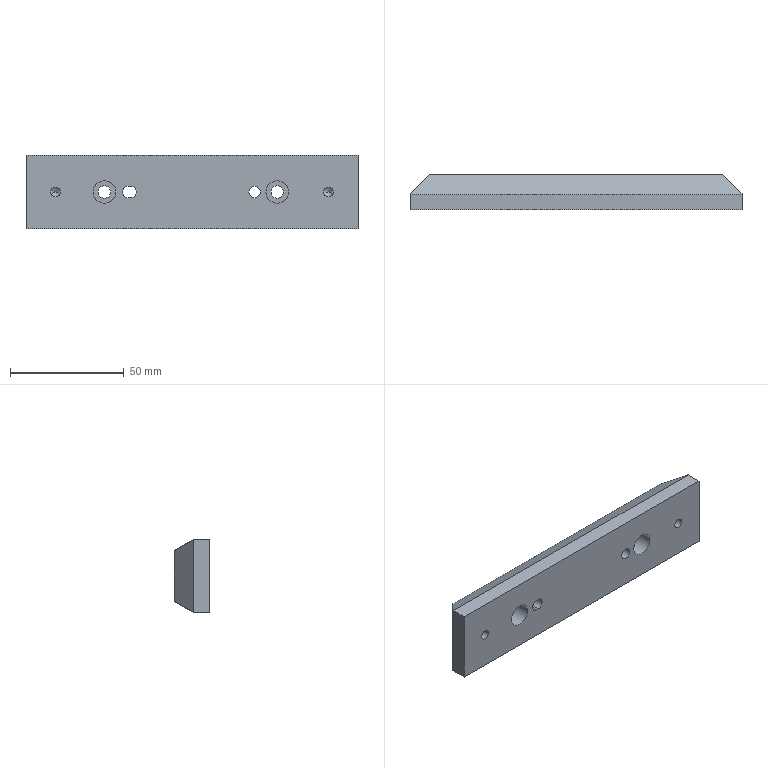Part | NX | 1 solid | 34 faces | box 146 x 15.5 x 32.5 mm | volume 62295 mm3 | cylinder 16 | plane 14 | cone 4 | commonest cylinder face diameters 4.2 x4 5 x4 5.5 x4 10 x4
STEP:
#1=CARTESIAN_POINT('',(73.,-7.75,-16.25));
#2=VERTEX_POINT('',#1);
#3=CARTESIAN_POINT('',(-73.,-7.75,-16.25));
#4=VERTEX_POINT('',#3);
#5=CARTESIAN_POINT('',(73.,-7.75,-16.25));
#6=DIRECTION('',(-1.,0.,0.));
#7=VECTOR('',#6,1000.);
#8=LINE('',#5,#7);
#9=EDGE_CURVE('',#2,#4,#8,.T.);
#10=ORIENTED_EDGE('',*,*,#9,.F.);
#11=CARTESIAN_POINT('',(73.,-7.75,16.25));
#12=VERTEX_POINT('',#11);
#13=CARTESIAN_POINT('',(73.,-7.75,16.25));
#14=DIRECTION('',(0.,0.,-1.));
#15=VECTOR('',#14,1000.);
#16=LINE('',#13,#15);
#17=EDGE_CURVE('',#12,#2,#16,.T.);
#18=ORIENTED_EDGE('',*,*,#17,.F.);
#19=CARTESIAN_POINT('',(-73.,-7.75,16.25));
#20=VERTEX_POINT('',#19);
#21=CARTESIAN_POINT('',(-73.,-7.75,16.25));
#22=DIRECTION('',(1.,0.,0.));
#23=VECTOR('',#22,1000.);
#24=LINE('',#21,#23);
#25=EDGE_CURVE('',#20,#12,#24,.T.);
#26=ORIENTED_EDGE('',*,*,#25,.F.);
#27=CARTESIAN_POINT('',(-73.,-7.75,-16.25));
#28=DIRECTION('',(0.,0.,1.));
#29=VECTOR('',#28,1000.);
#30=LINE('',#27,#29);
#31=EDGE_CURVE('',#4,#20,#30,.T.);
#32=ORIENTED_EDGE('',*,*,#31,.F.);
#33=EDGE_LOOP('',(#10,#18,#26,#32));
#34=FACE_BOUND('',#33,.T.);
#35=CARTESIAN_POINT('',(42.5,-7.75,0.));
#36=VERTEX_POINT('',#35);
#37=CARTESIAN_POINT('',(32.5,-7.75,0.));
#38=VERTEX_POINT('',#37);
#39=CARTESIAN_POINT('',(37.5,-7.75,0.));
#40=DIRECTION('',(0.,-1.,0.));
#41=DIRECTION('',(1.,0.,0.));
#42=AXIS2_PLACEMENT_3D('',#39,#40,#41);
#43=CIRCLE('',#42,5.);
#44=EDGE_CURVE('',#36,#38,#43,.T.);
#45=ORIENTED_EDGE('',*,*,#44,.F.);
#46=CARTESIAN_POINT('',(37.5,-7.75,0.));
#47=DIRECTION('',(0.,-1.,0.));
#48=DIRECTION('',(-1.,0.,0.));
#49=AXIS2_PLACEMENT_3D('',#46,#47,#48);
#50=CIRCLE('',#49,5.);
#51=EDGE_CURVE('',#38,#36,#50,.T.);
#52=ORIENTED_EDGE('',*,*,#51,.F.);
#53=EDGE_LOOP('',(#45,#52));
#54=FACE_BOUND('',#53,.T.);
#55=CARTESIAN_POINT('',(-33.5,-7.75,0.));
#56=VERTEX_POINT('',#55);
#57=CARTESIAN_POINT('',(-43.5,-7.75,0.));
#58=VERTEX_POINT('',#57);
#59=CARTESIAN_POINT('',(-38.5,-7.75,0.));
#60=DIRECTION('',(0.,-1.,0.));
#61=DIRECTION('',(1.,0.,0.));
#62=AXIS2_PLACEMENT_3D('',#59,#60,#61);
#63=CIRCLE('',#62,5.);
#64=EDGE_CURVE('',#56,#58,#63,.T.);
#65=ORIENTED_EDGE('',*,*,#64,.F.);
#66=CARTESIAN_POINT('',(-38.5,-7.75,0.));
#67=DIRECTION('',(0.,-1.,0.));
#68=DIRECTION('',(-1.,0.,0.));
#69=AXIS2_PLACEMENT_3D('',#66,#67,#68);
#70=CIRCLE('',#69,5.);
#71=EDGE_CURVE('',#58,#56,#70,.T.);
#72=ORIENTED_EDGE('',*,*,#71,.F.);
#73=EDGE_LOOP('',(#65,#72));
#74=FACE_BOUND('',#73,.T.);
#75=CARTESIAN_POINT('',(30.,-7.75,0.));
#76=VERTEX_POINT('',#75);
#77=CARTESIAN_POINT('',(25.,-7.75,0.));
#78=VERTEX_POINT('',#77);
#79=CARTESIAN_POINT('',(27.5,-7.75,0.));
#80=DIRECTION('',(0.,-1.,0.));
#81=DIRECTION('',(1.,0.,0.));
#82=AXIS2_PLACEMENT_3D('',#79,#80,#81);
#83=CIRCLE('',#82,2.5);
#84=EDGE_CURVE('',#76,#78,#83,.T.);
#85=ORIENTED_EDGE('',*,*,#84,.F.);
#86=CARTESIAN_POINT('',(27.5,-7.75,0.));
#87=DIRECTION('',(0.,-1.,0.));
#88=DIRECTION('',(-1.,0.,0.));
#89=AXIS2_PLACEMENT_3D('',#86,#87,#88);
#90=CIRCLE('',#89,2.5);
#91=EDGE_CURVE('',#78,#76,#90,.T.);
#92=ORIENTED_EDGE('',*,*,#91,.F.);
#93=EDGE_LOOP('',(#85,#92));
#94=FACE_BOUND('',#93,.T.);
#95=CARTESIAN_POINT('',(-28.,-7.75,-2.5));
#96=VERTEX_POINT('',#95);
#97=CARTESIAN_POINT('',(-27.,-7.75,-2.5));
#98=VERTEX_POINT('',#97);
#99=CARTESIAN_POINT('',(-28.,-7.75,-2.5));
#100=DIRECTION('',(1.,0.,0.));
#101=VECTOR('',#100,1000.);
#102=LINE('',#99,#101);
#103=EDGE_CURVE('',#96,#98,#102,.T.);
#104=ORIENTED_EDGE('',*,*,#103,.F.);
#105=CARTESIAN_POINT('',(-28.,-7.75,2.5));
#106=VERTEX_POINT('',#105);
#107=CARTESIAN_POINT('',(-28.,-7.75,0.));
#108=DIRECTION('',(0.,-1.,0.));
#109=DIRECTION('',(0.,0.,1.));
#110=AXIS2_PLACEMENT_3D('',#107,#108,#109);
#111=CIRCLE('',#110,2.5);
#112=EDGE_CURVE('',#106,#96,#111,.T.);
#113=ORIENTED_EDGE('',*,*,#112,.F.);
#114=CARTESIAN_POINT('',(-27.,-7.75,2.5));
#115=VERTEX_POINT('',#114);
#116=CARTESIAN_POINT('',(-27.,-7.75,2.5));
#117=DIRECTION('',(-1.,0.,0.));
#118=VECTOR('',#117,1000.);
#119=LINE('',#116,#118);
#120=EDGE_CURVE('',#115,#106,#119,.T.);
#121=ORIENTED_EDGE('',*,*,#120,.F.);
#122=CARTESIAN_POINT('',(-27.,-7.75,0.));
#123=DIRECTION('',(0.,-1.,0.));
#124=DIRECTION('',(0.,0.,-1.));
#125=AXIS2_PLACEMENT_3D('',#122,#123,#124);
#126=CIRCLE('',#125,2.5);
#127=EDGE_CURVE('',#98,#115,#126,.T.);
#128=ORIENTED_EDGE('',*,*,#127,.F.);
#129=EDGE_LOOP('',(#104,#113,#121,#128));
#130=FACE_BOUND('',#129,.T.);
#131=CARTESIAN_POINT('',(62.1,-7.75,0.));
#132=VERTEX_POINT('',#131);
#133=CARTESIAN_POINT('',(57.9,-7.75,0.));
#134=VERTEX_POINT('',#133);
#135=CARTESIAN_POINT('',(60.,-7.75,0.));
#136=DIRECTION('',(0.,-1.,0.));
#137=DIRECTION('',(1.,0.,0.));
#138=AXIS2_PLACEMENT_3D('',#135,#136,#137);
#139=CIRCLE('',#138,2.1);
#140=EDGE_CURVE('',#132,#134,#139,.T.);
#141=ORIENTED_EDGE('',*,*,#140,.F.);
#142=CARTESIAN_POINT('',(60.,-7.75,0.));
#143=DIRECTION('',(0.,-1.,0.));
#144=DIRECTION('',(-1.,0.,0.));
#145=AXIS2_PLACEMENT_3D('',#142,#143,#144);
#146=CIRCLE('',#145,2.1);
#147=EDGE_CURVE('',#134,#132,#146,.T.);
#148=ORIENTED_EDGE('',*,*,#147,.F.);
#149=EDGE_LOOP('',(#141,#148));
#150=FACE_BOUND('',#149,.T.);
#151=CARTESIAN_POINT('',(-57.9,-7.75,0.));
#152=VERTEX_POINT('',#151);
#153=CARTESIAN_POINT('',(-62.1,-7.75,0.));
#154=VERTEX_POINT('',#153);
#155=CARTESIAN_POINT('',(-60.,-7.75,0.));
#156=DIRECTION('',(0.,-1.,0.));
#157=DIRECTION('',(1.,0.,0.));
#158=AXIS2_PLACEMENT_3D('',#155,#156,#157);
#159=CIRCLE('',#158,2.1);
#160=EDGE_CURVE('',#152,#154,#159,.T.);
#161=ORIENTED_EDGE('',*,*,#160,.F.);
#162=CARTESIAN_POINT('',(-60.,-7.75,0.));
#163=DIRECTION('',(0.,-1.,0.));
#164=DIRECTION('',(-1.,0.,0.));
#165=AXIS2_PLACEMENT_3D('',#162,#163,#164);
#166=CIRCLE('',#165,2.1);
#167=EDGE_CURVE('',#154,#152,#166,.T.);
#168=ORIENTED_EDGE('',*,*,#167,.F.);
#169=EDGE_LOOP('',(#161,#168));
#170=FACE_BOUND('',#169,.T.);
#171=CARTESIAN_POINT('',(0.,-7.75,0.));
#172=DIRECTION('',(0.,1.,0.));
#173=DIRECTION('',(-1.,0.,0.));
#174=AXIS2_PLACEMENT_3D('',#171,#172,#173);
#175=PLANE('',#174);
#176=ADVANCED_FACE('',(#34,#54,#74,#94,#130,#150,#170),#175,.F.);
#177=CARTESIAN_POINT('',(-73.,-0.7571,-16.084));
#178=VERTEX_POINT('',#177);
#179=CARTESIAN_POINT('',(-73.,-1.044,-16.25));
#180=VERTEX_POINT('',#179);
#181=CARTESIAN_POINT('',(-73.,-0.7571,-16.084));
#182=DIRECTION('',(0.,-0.866,-0.5));
#183=VECTOR('',#182,1000.);
#184=LINE('',#181,#183);
#185=EDGE_CURVE('',#178,#180,#184,.T.);
#186=ORIENTED_EDGE('',*,*,#185,.T.);
#187=CARTESIAN_POINT('',(-73.,-7.75,-16.25));
#188=DIRECTION('',(0.,1.,0.));
#189=VECTOR('',#188,1000.);
#190=LINE('',#187,#189);
#191=EDGE_CURVE('',#4,#180,#190,.T.);
#192=ORIENTED_EDGE('',*,*,#191,.F.);
#193=ORIENTED_EDGE('',*,*,#31,.T.);
#194=CARTESIAN_POINT('',(-73.,-1.044,16.25));
#195=VERTEX_POINT('',#194);
#196=CARTESIAN_POINT('',(-73.,-7.75,16.25));
#197=DIRECTION('',(0.,1.,0.));
#198=VECTOR('',#197,1000.);
#199=LINE('',#196,#198);
#200=EDGE_CURVE('',#20,#195,#199,.T.);
#201=ORIENTED_EDGE('',*,*,#200,.T.);
#202=CARTESIAN_POINT('',(-73.,-0.7571,16.084));
#203=VERTEX_POINT('',#202);
#204=CARTESIAN_POINT('',(-73.,-1.044,16.25));
#205=DIRECTION('',(0.,0.866,-0.5));
#206=VECTOR('',#205,1000.);
#207=LINE('',#204,#206);
#208=EDGE_CURVE('',#195,#203,#207,.T.);
#209=ORIENTED_EDGE('',*,*,#208,.T.);
#210=CARTESIAN_POINT('',(-73.,-0.7571,-16.084));
#211=DIRECTION('',(0.,0.,1.));
#212=VECTOR('',#211,1000.);
#213=LINE('',#210,#212);
#214=EDGE_CURVE('',#178,#203,#213,.T.);
#215=ORIENTED_EDGE('',*,*,#214,.F.);
#216=EDGE_LOOP('',(#186,#192,#193,#201,#209,#215));
#217=FACE_BOUND('',#216,.T.);
#218=CARTESIAN_POINT('',(-73.,-7.75,-16.25));
#219=DIRECTION('',(-1.,0.,0.));
#220=DIRECTION('',(0.,0.,-1.));
#221=AXIS2_PLACEMENT_3D('',#218,#219,#220);
#222=PLANE('',#221);
#223=ADVANCED_FACE('',(#217),#222,.T.);
#224=CARTESIAN_POINT('',(-64.493,7.75,-11.173));
#225=VERTEX_POINT('',#224);
#226=CARTESIAN_POINT('',(-73.,-0.7571,-16.084));
#227=DIRECTION('',(0.6547,0.6547,0.378));
#228=VECTOR('',#227,1000.);
#229=LINE('',#226,#228);
#230=EDGE_CURVE('',#178,#225,#229,.T.);
#231=ORIENTED_EDGE('',*,*,#230,.F.);
#232=ORIENTED_EDGE('',*,*,#214,.T.);
#233=CARTESIAN_POINT('',(-64.493,7.75,11.173));
#234=VERTEX_POINT('',#233);
#235=CARTESIAN_POINT('',(-73.,-0.7571,16.084));
#236=DIRECTION('',(0.6547,0.6547,-0.378));
#237=VECTOR('',#236,1000.);
#238=LINE('',#235,#237);
#239=EDGE_CURVE('',#203,#234,#238,.T.);
#240=ORIENTED_EDGE('',*,*,#239,.T.);
#241=CARTESIAN_POINT('',(-64.493,7.75,11.173));
#242=DIRECTION('',(0.,0.,-1.));
#243=VECTOR('',#242,1000.);
#244=LINE('',#241,#243);
#245=EDGE_CURVE('',#234,#225,#244,.T.);
#246=ORIENTED_EDGE('',*,*,#245,.T.);
#247=EDGE_LOOP('',(#231,#232,#240,#246));
#248=FACE_BOUND('',#247,.T.);
#249=CARTESIAN_POINT('',(-75.488,-3.245,-19.5));
#250=DIRECTION('',(0.7071,-0.7071,0.));
#251=DIRECTION('',(-0.7071,-0.7071,0.));
#252=AXIS2_PLACEMENT_3D('',#249,#250,#251);
#253=PLANE('',#252);
#254=ADVANCED_FACE('',(#248),#253,.F.);
#255=CARTESIAN_POINT('',(64.493,7.75,-11.173));
#256=VERTEX_POINT('',#255);
#257=CARTESIAN_POINT('',(-64.493,7.75,-11.173));
#258=DIRECTION('',(1.,0.,0.));
#259=VECTOR('',#258,1000.);
#260=LINE('',#257,#259);
#261=EDGE_CURVE('',#225,#256,#260,.T.);
#262=ORIENTED_EDGE('',*,*,#261,.F.);
#263=ORIENTED_EDGE('',*,*,#245,.F.);
#264=CARTESIAN_POINT('',(64.493,7.75,11.173));
#265=VERTEX_POINT('',#264);
#266=CARTESIAN_POINT('',(-64.493,7.75,11.173));
#267=DIRECTION('',(1.,0.,0.));
#268=VECTOR('',#267,1000.);
#269=LINE('',#266,#268);
#270=EDGE_CURVE('',#234,#265,#269,.T.);
#271=ORIENTED_EDGE('',*,*,#270,.T.);
#272=CARTESIAN_POINT('',(64.493,7.75,11.173));
#273=DIRECTION('',(0.,0.,-1.));
#274=VECTOR('',#273,1000.);
#275=LINE('',#272,#274);
#276=EDGE_CURVE('',#265,#256,#275,.T.);
#277=ORIENTED_EDGE('',*,*,#276,.T.);
#278=EDGE_LOOP('',(#262,#263,#271,#277));
#279=FACE_BOUND('',#278,.T.);
#280=CARTESIAN_POINT('',(-35.75,7.75,0.));
#281=VERTEX_POINT('',#280);
#282=CARTESIAN_POINT('',(-41.25,7.75,0.));
#283=VERTEX_POINT('',#282);
#284=CARTESIAN_POINT('',(-38.5,7.75,0.));
#285=DIRECTION('',(0.,-1.,0.));
#286=DIRECTION('',(1.,0.,0.));
#287=AXIS2_PLACEMENT_3D('',#284,#285,#286);
#288=CIRCLE('',#287,2.75);
#289=EDGE_CURVE('',#281,#283,#288,.T.);
#290=ORIENTED_EDGE('',*,*,#289,.T.);
#291=CARTESIAN_POINT('',(-38.5,7.75,0.));
#292=DIRECTION('',(0.,-1.,0.));
#293=DIRECTION('',(-1.,0.,0.));
#294=AXIS2_PLACEMENT_3D('',#291,#292,#293);
#295=CIRCLE('',#294,2.75);
#296=EDGE_CURVE('',#283,#281,#295,.T.);
#297=ORIENTED_EDGE('',*,*,#296,.T.);
#298=EDGE_LOOP('',(#290,#297));
#299=FACE_BOUND('',#298,.T.);
#300=CARTESIAN_POINT('',(30.,7.75,0.));
#301=VERTEX_POINT('',#300);
#302=CARTESIAN_POINT('',(25.,7.75,0.));
#303=VERTEX_POINT('',#302);
#304=CARTESIAN_POINT('',(27.5,7.75,0.));
#305=DIRECTION('',(0.,-1.,0.));
#306=DIRECTION('',(1.,0.,0.));
#307=AXIS2_PLACEMENT_3D('',#304,#305,#306);
#308=CIRCLE('',#307,2.5);
#309=EDGE_CURVE('',#301,#303,#308,.T.);
#310=ORIENTED_EDGE('',*,*,#309,.T.);
#311=CARTESIAN_POINT('',(27.5,7.75,0.));
#312=DIRECTION('',(0.,-1.,0.));
#313=DIRECTION('',(-1.,0.,0.));
#314=AXIS2_PLACEMENT_3D('',#311,#312,#313);
#315=CIRCLE('',#314,2.5);
#316=EDGE_CURVE('',#303,#301,#315,.T.);
#317=ORIENTED_EDGE('',*,*,#316,.T.);
#318=EDGE_LOOP('',(#310,#317));
#319=FACE_BOUND('',#318,.T.);
#320=CARTESIAN_POINT('',(-28.,7.75,2.5));
#321=VERTEX_POINT('',#320);
#322=CARTESIAN_POINT('',(-27.,7.75,2.5));
#323=VERTEX_POINT('',#322);
#324=CARTESIAN_POINT('',(-28.,7.75,2.5));
#325=DIRECTION('',(1.,0.,0.));
#326=VECTOR('',#325,1000.);
#327=LINE('',#324,#326);
#328=EDGE_CURVE('',#321,#323,#327,.T.);
#329=ORIENTED_EDGE('',*,*,#328,.F.);
#330=CARTESIAN_POINT('',(-28.,7.75,-2.5));
#331=VERTEX_POINT('',#330);
#332=CARTESIAN_POINT('',(-28.,7.75,0.));
#333=DIRECTION('',(0.,-1.,0.));
#334=DIRECTION('',(0.,0.,1.));
#335=AXIS2_PLACEMENT_3D('',#332,#333,#334);
#336=CIRCLE('',#335,2.5);
#337=EDGE_CURVE('',#321,#331,#336,.T.);
#338=ORIENTED_EDGE('',*,*,#337,.T.);
#339=CARTESIAN_POINT('',(-27.,7.75,-2.5));
#340=VERTEX_POINT('',#339);
#341=CARTESIAN_POINT('',(-27.,7.75,-2.5));
#342=DIRECTION('',(-1.,0.,0.));
#343=VECTOR('',#342,1000.);
#344=LINE('',#341,#343);
#345=EDGE_CURVE('',#340,#331,#344,.T.);
#346=ORIENTED_EDGE('',*,*,#345,.F.);
#347=CARTESIAN_POINT('',(-27.,7.75,0.));
#348=DIRECTION('',(0.,-1.,0.));
#349=DIRECTION('',(0.,0.,-1.));
#350=AXIS2_PLACEMENT_3D('',#347,#348,#349);
#351=CIRCLE('',#350,2.5);
#352=EDGE_CURVE('',#340,#323,#351,.T.);
#353=ORIENTED_EDGE('',*,*,#352,.T.);
#354=EDGE_LOOP('',(#329,#338,#346,#353));
#355=FACE_BOUND('',#354,.T.);
#356=CARTESIAN_POINT('',(40.25,7.75,0.));
#357=VERTEX_POINT('',#356);
#358=CARTESIAN_POINT('',(34.75,7.75,0.));
#359=VERTEX_POINT('',#358);
#360=CARTESIAN_POINT('',(37.5,7.75,0.));
#361=DIRECTION('',(0.,-1.,0.));
#362=DIRECTION('',(1.,0.,0.));
#363=AXIS2_PLACEMENT_3D('',#360,#361,#362);
#364=CIRCLE('',#363,2.75);
#365=EDGE_CURVE('',#357,#359,#364,.T.);
#366=ORIENTED_EDGE('',*,*,#365,.T.);
#367=CARTESIAN_POINT('',(37.5,7.75,0.));
#368=DIRECTION('',(0.,-1.,0.));
#369=DIRECTION('',(-1.,0.,0.));
#370=AXIS2_PLACEMENT_3D('',#367,#368,#369);
#371=CIRCLE('',#370,2.75);
#372=EDGE_CURVE('',#359,#357,#371,.T.);
#373=ORIENTED_EDGE('',*,*,#372,.T.);
#374=EDGE_LOOP('',(#366,#373));
#375=FACE_BOUND('',#374,.T.);
#376=CARTESIAN_POINT('',(0.,7.75,0.));
#377=DIRECTION('',(0.,1.,0.));
#378=DIRECTION('',(-1.,0.,0.));
#379=AXIS2_PLACEMENT_3D('',#376,#377,#378);
#380=PLANE('',#379);
#381=ADVANCED_FACE('',(#279,#299,#319,#355,#375),#380,.T.);
#382=CARTESIAN_POINT('',(34.75,2.25,0.));
#383=VERTEX_POINT('',#382);
#384=CARTESIAN_POINT('',(40.25,2.25,0.));
#385=VERTEX_POINT('',#384);
#386=CARTESIAN_POINT('',(37.5,2.25,0.));
#387=DIRECTION('',(0.,-1.,0.));
#388=DIRECTION('',(-1.,0.,0.));
#389=AXIS2_PLACEMENT_3D('',#386,#387,#388);
#390=CIRCLE('',#389,2.75);
#391=EDGE_CURVE('',#383,#385,#390,.T.);
#392=ORIENTED_EDGE('',*,*,#391,.T.);
#393=CARTESIAN_POINT('',(40.25,7.75,0.));
#394=DIRECTION('',(0.,-1.,0.));
#395=VECTOR('',#394,1000.);
#396=LINE('',#393,#395);
#397=EDGE_CURVE('',#357,#385,#396,.T.);
#398=ORIENTED_EDGE('',*,*,#397,.F.);
#399=ORIENTED_EDGE('',*,*,#372,.F.);
#400=CARTESIAN_POINT('',(34.75,7.75,0.));
#401=DIRECTION('',(0.,-1.,0.));
#402=VECTOR('',#401,1000.);
#403=LINE('',#400,#402);
#404=EDGE_CURVE('',#359,#383,#403,.T.);
#405=ORIENTED_EDGE('',*,*,#404,.T.);
#406=EDGE_LOOP('',(#392,#398,#399,#405));
#407=FACE_BOUND('',#406,.T.);
#408=CARTESIAN_POINT('',(37.5,10.152,0.));
#409=DIRECTION('',(0.,-1.,0.));
#410=DIRECTION('',(1.,0.,0.));
#411=AXIS2_PLACEMENT_3D('',#408,#409,#410);
#412=CYLINDRICAL_SURFACE('',#411,2.75);
#413=ADVANCED_FACE('',(#407),#412,.F.);
#414=ORIENTED_EDGE('',*,*,#365,.F.);
#415=ORIENTED_EDGE('',*,*,#397,.T.);
#416=CARTESIAN_POINT('',(37.5,2.25,0.));
#417=DIRECTION('',(0.,1.,0.));
#418=DIRECTION('',(-1.,0.,0.));
#419=AXIS2_PLACEMENT_3D('',#416,#417,#418);
#420=CIRCLE('',#419,2.75);
#421=EDGE_CURVE('',#383,#385,#420,.T.);
#422=ORIENTED_EDGE('',*,*,#421,.F.);
#423=ORIENTED_EDGE('',*,*,#404,.F.);
#424=EDGE_LOOP('',(#414,#415,#422,#423));
#425=FACE_BOUND('',#424,.T.);
#426=CARTESIAN_POINT('',(37.5,10.152,0.));
#427=DIRECTION('',(0.,-1.,0.));
#428=DIRECTION('',(1.,0.,0.));
#429=AXIS2_PLACEMENT_3D('',#426,#427,#428);
#430=CYLINDRICAL_SURFACE('',#429,2.75);
#431=ADVANCED_FACE('',(#425),#430,.F.);
#432=CARTESIAN_POINT('',(32.5,2.25,0.));
#433=VERTEX_POINT('',#432);
#434=CARTESIAN_POINT('',(42.5,2.25,0.));
#435=VERTEX_POINT('',#434);
#436=CARTESIAN_POINT('',(37.5,2.25,0.));
#437=DIRECTION('',(0.,1.,0.));
#438=DIRECTION('',(-1.,0.,0.));
#439=AXIS2_PLACEMENT_3D('',#436,#437,#438);
#440=CIRCLE('',#439,5.);
#441=EDGE_CURVE('',#433,#435,#440,.T.);
#442=ORIENTED_EDGE('',*,*,#441,.F.);
#443=CARTESIAN_POINT('',(37.5,2.25,0.));
#444=DIRECTION('',(0.,-1.,0.));
#445=DIRECTION('',(-1.,0.,0.));
#446=AXIS2_PLACEMENT_3D('',#443,#444,#445);
#447=CIRCLE('',#446,5.);
#448=EDGE_CURVE('',#433,#435,#447,.T.);
#449=ORIENTED_EDGE('',*,*,#448,.T.);
#450=EDGE_LOOP('',(#442,#449));
#451=FACE_BOUND('',#450,.T.);
#452=ORIENTED_EDGE('',*,*,#391,.F.);
#453=ORIENTED_EDGE('',*,*,#421,.T.);
#454=EDGE_LOOP('',(#452,#453));
#455=FACE_BOUND('',#454,.T.);
#456=CARTESIAN_POINT('',(37.5,2.25,0.));
#457=DIRECTION('',(0.,-1.,0.));
#458=DIRECTION('',(1.,0.,0.));
#459=AXIS2_PLACEMENT_3D('',#456,#457,#458);
#460=PLANE('',#459);
#461=ADVANCED_FACE('',(#451,#455),#460,.T.);
#462=CARTESIAN_POINT('',(42.5,2.25,0.));
#463=DIRECTION('',(0.,-1.,0.));
#464=VECTOR('',#463,1000.);
#465=LINE('',#462,#464);
#466=EDGE_CURVE('',#435,#36,#465,.T.);
#467=ORIENTED_EDGE('',*,*,#466,.F.);
#468=ORIENTED_EDGE('',*,*,#448,.F.);
#469=CARTESIAN_POINT('',(32.5,2.25,0.));
#470=DIRECTION('',(0.,-1.,0.));
#471=VECTOR('',#470,1000.);
#472=LINE('',#469,#471);
#473=EDGE_CURVE('',#433,#38,#472,.T.);
#474=ORIENTED_EDGE('',*,*,#473,.T.);
#475=ORIENTED_EDGE('',*,*,#51,.T.);
#476=EDGE_LOOP('',(#467,#468,#474,#475));
#477=FACE_BOUND('',#476,.T.);
#478=CARTESIAN_POINT('',(37.5,10.152,0.));
#479=DIRECTION('',(0.,-1.,0.));
#480=DIRECTION('',(1.,0.,0.));
#481=AXIS2_PLACEMENT_3D('',#478,#479,#480);
#482=CYLINDRICAL_SURFACE('',#481,5.);
#483=ADVANCED_FACE('',(#477),#482,.F.);
#484=ORIENTED_EDGE('',*,*,#473,.F.);
#485=ORIENTED_EDGE('',*,*,#441,.T.);
#486=ORIENTED_EDGE('',*,*,#466,.T.);
#487=ORIENTED_EDGE('',*,*,#44,.T.);
#488=EDGE_LOOP('',(#484,#485,#486,#487));
#489=FACE_BOUND('',#488,.T.);
#490=CARTESIAN_POINT('',(37.5,10.152,0.));
#491=DIRECTION('',(0.,-1.,0.));
#492=DIRECTION('',(1.,0.,0.));
#493=AXIS2_PLACEMENT_3D('',#490,#491,#492);
#494=CYLINDRICAL_SURFACE('',#493,5.);
#495=ADVANCED_FACE('',(#489),#494,.F.);
#496=CARTESIAN_POINT('',(-41.25,2.25,0.));
#497=VERTEX_POINT('',#496);
#498=CARTESIAN_POINT('',(-35.75,2.25,0.));
#499=VERTEX_POINT('',#498);
#500=CARTESIAN_POINT('',(-38.5,2.25,0.));
#501=DIRECTION('',(0.,-1.,0.));
#502=DIRECTION('',(-1.,0.,0.));
#503=AXIS2_PLACEMENT_3D('',#500,#501,#502);
#504=CIRCLE('',#503,2.75);
#505=EDGE_CURVE('',#497,#499,#504,.T.);
#506=ORIENTED_EDGE('',*,*,#505,.T.);
#507=CARTESIAN_POINT('',(-35.75,7.75,0.));
#508=DIRECTION('',(0.,-1.,0.));
#509=VECTOR('',#508,1000.);
#510=LINE('',#507,#509);
#511=EDGE_CURVE('',#281,#499,#510,.T.);
#512=ORIENTED_EDGE('',*,*,#511,.F.);
#513=ORIENTED_EDGE('',*,*,#296,.F.);
#514=CARTESIAN_POINT('',(-41.25,7.75,0.));
#515=DIRECTION('',(0.,-1.,0.));
#516=VECTOR('',#515,1000.);
#517=LINE('',#514,#516);
#518=EDGE_CURVE('',#283,#497,#517,.T.);
#519=ORIENTED_EDGE('',*,*,#518,.T.);
#520=EDGE_LOOP('',(#506,#512,#513,#519));
#521=FACE_BOUND('',#520,.T.);
#522=CARTESIAN_POINT('',(-38.5,10.152,0.));
#523=DIRECTION('',(0.,-1.,0.));
#524=DIRECTION('',(1.,0.,0.));
#525=AXIS2_PLACEMENT_3D('',#522,#523,#524);
#526=CYLINDRICAL_SURFACE('',#525,2.75);
#527=ADVANCED_FACE('',(#521),#526,.F.);
#528=ORIENTED_EDGE('',*,*,#289,.F.);
#529=ORIENTED_EDGE('',*,*,#511,.T.);
#530=CARTESIAN_POINT('',(-38.5,2.25,0.));
#531=DIRECTION('',(0.,1.,0.));
#532=DIRECTION('',(-1.,0.,0.));
#533=AXIS2_PLACEMENT_3D('',#530,#531,#532);
#534=CIRCLE('',#533,2.75);
#535=EDGE_CURVE('',#497,#499,#534,.T.);
#536=ORIENTED_EDGE('',*,*,#535,.F.);
#537=ORIENTED_EDGE('',*,*,#518,.F.);
#538=EDGE_LOOP('',(#528,#529,#536,#537));
#539=FACE_BOUND('',#538,.T.);
#540=CARTESIAN_POINT('',(-38.5,10.152,0.));
#541=DIRECTION('',(0.,-1.,0.));
#542=DIRECTION('',(1.,0.,0.));
#543=AXIS2_PLACEMENT_3D('',#540,#541,#542);
#544=CYLINDRICAL_SURFACE('',#543,2.75);
#545=ADVANCED_FACE('',(#539),#544,.F.);
#546=CARTESIAN_POINT('',(-43.5,2.25,0.));
#547=VERTEX_POINT('',#546);
#548=CARTESIAN_POINT('',(-33.5,2.25,0.));
#549=VERTEX_POINT('',#548);
#550=CARTESIAN_POINT('',(-38.5,2.25,0.));
#551=DIRECTION('',(0.,1.,0.));
#552=DIRECTION('',(-1.,0.,0.));
#553=AXIS2_PLACEMENT_3D('',#550,#551,#552);
#554=CIRCLE('',#553,5.);
#555=EDGE_CURVE('',#547,#549,#554,.T.);
#556=ORIENTED_EDGE('',*,*,#555,.F.);
#557=CARTESIAN_POINT('',(-38.5,2.25,0.));
#558=DIRECTION('',(0.,-1.,0.));
#559=DIRECTION('',(-1.,0.,0.));
#560=AXIS2_PLACEMENT_3D('',#557,#558,#559);
#561=CIRCLE('',#560,5.);
#562=EDGE_CURVE('',#547,#549,#561,.T.);
#563=ORIENTED_EDGE('',*,*,#562,.T.);
#564=EDGE_LOOP('',(#556,#563));
#565=FACE_BOUND('',#564,.T.);
#566=ORIENTED_EDGE('',*,*,#505,.F.);
#567=ORIENTED_EDGE('',*,*,#535,.T.);
#568=EDGE_LOOP('',(#566,#567));
#569=FACE_BOUND('',#568,.T.);
#570=CARTESIAN_POINT('',(-38.5,2.25,0.));
#571=DIRECTION('',(0.,-1.,0.));
#572=DIRECTION('',(1.,0.,0.));
#573=AXIS2_PLACEMENT_3D('',#570,#571,#572);
#574=PLANE('',#573);
#575=ADVANCED_FACE('',(#565,#569),#574,.T.);
#576=CARTESIAN_POINT('',(-33.5,2.25,0.));
#577=DIRECTION('',(0.,-1.,0.));
#578=VECTOR('',#577,1000.);
#579=LINE('',#576,#578);
#580=EDGE_CURVE('',#549,#56,#579,.T.);
#581=ORIENTED_EDGE('',*,*,#580,.F.);
#582=ORIENTED_EDGE('',*,*,#562,.F.);
#583=CARTESIAN_POINT('',(-43.5,2.25,0.));
#584=DIRECTION('',(0.,-1.,0.));
#585=VECTOR('',#584,1000.);
#586=LINE('',#583,#585);
#587=EDGE_CURVE('',#547,#58,#586,.T.);
#588=ORIENTED_EDGE('',*,*,#587,.T.);
#589=ORIENTED_EDGE('',*,*,#71,.T.);
#590=EDGE_LOOP('',(#581,#582,#588,#589));
#591=FACE_BOUND('',#590,.T.);
#592=CARTESIAN_POINT('',(-38.5,10.152,0.));
#593=DIRECTION('',(0.,-1.,0.));
#594=DIRECTION('',(1.,0.,0.));
#595=AXIS2_PLACEMENT_3D('',#592,#593,#594);
#596=CYLINDRICAL_SURFACE('',#595,5.);
#597=ADVANCED_FACE('',(#591),#596,.F.);
#598=ORIENTED_EDGE('',*,*,#587,.F.);
#599=ORIENTED_EDGE('',*,*,#555,.T.);
#600=ORIENTED_EDGE('',*,*,#580,.T.);
#601=ORIENTED_EDGE('',*,*,#64,.T.);
#602=EDGE_LOOP('',(#598,#599,#600,#601));
#603=FACE_BOUND('',#602,.T.);
#604=CARTESIAN_POINT('',(-38.5,10.152,0.));
#605=DIRECTION('',(0.,-1.,0.));
#606=DIRECTION('',(1.,0.,0.));
#607=AXIS2_PLACEMENT_3D('',#604,#605,#606);
#608=CYLINDRICAL_SURFACE('',#607,5.);
#609=ADVANCED_FACE('',(#603),#608,.F.);
#610=CARTESIAN_POINT('',(30.,-7.75,0.));
#611=DIRECTION('',(0.,1.,0.));
#612=VECTOR('',#611,1000.);
#613=LINE('',#610,#612);
#614=EDGE_CURVE('',#76,#301,#613,.T.);
#615=ORIENTED_EDGE('',*,*,#614,.T.);
#616=ORIENTED_EDGE('',*,*,#316,.F.);
#617=CARTESIAN_POINT('',(25.,-7.75,0.));
#618=DIRECTION('',(0.,1.,0.));
#619=VECTOR('',#618,1000.);
#620=LINE('',#617,#619);
#621=EDGE_CURVE('',#78,#303,#620,.T.);
#622=ORIENTED_EDGE('',*,*,#621,.F.);
#623=ORIENTED_EDGE('',*,*,#91,.T.);
#624=EDGE_LOOP('',(#615,#616,#622,#623));
#625=FACE_BOUND('',#624,.T.);
#626=CARTESIAN_POINT('',(27.5,-7.75,0.));
#627=DIRECTION('',(0.,-1.,0.));
#628=DIRECTION('',(1.,0.,0.));
#629=AXIS2_PLACEMENT_3D('',#626,#627,#628);
#630=CYLINDRICAL_SURFACE('',#629,2.5);
#631=ADVANCED_FACE('',(#625),#630,.F.);
#632=ORIENTED_EDGE('',*,*,#621,.T.);
#633=ORIENTED_EDGE('',*,*,#309,.F.);
#634=ORIENTED_EDGE('',*,*,#614,.F.);
#635=ORIENTED_EDGE('',*,*,#84,.T.);
#636=EDGE_LOOP('',(#632,#633,#634,#635));
#637=FACE_BOUND('',#636,.T.);
#638=CARTESIAN_POINT('',(27.5,-7.75,0.));
#639=DIRECTION('',(0.,-1.,0.));
#640=DIRECTION('',(1.,0.,0.));
#641=AXIS2_PLACEMENT_3D('',#638,#639,#640);
#642=CYLINDRICAL_SURFACE('',#641,2.5);
#643=ADVANCED_FACE('',(#637),#642,.F.);
#644=CARTESIAN_POINT('',(-27.,-7.75,2.5));
#645=DIRECTION('',(0.,1.,0.));
#646=VECTOR('',#645,1000.);
#647=LINE('',#644,#646);
#648=EDGE_CURVE('',#115,#323,#647,.T.);
#649=ORIENTED_EDGE('',*,*,#648,.T.);
#650=ORIENTED_EDGE('',*,*,#352,.F.);
#651=CARTESIAN_POINT('',(-27.,-7.75,-2.5));
#652=DIRECTION('',(0.,1.,0.));
#653=VECTOR('',#652,1000.);
#654=LINE('',#651,#653);
#655=EDGE_CURVE('',#98,#340,#654,.T.);
#656=ORIENTED_EDGE('',*,*,#655,.F.);
#657=ORIENTED_EDGE('',*,*,#127,.T.);
#658=EDGE_LOOP('',(#649,#650,#656,#657));
#659=FACE_BOUND('',#658,.T.);
#660=CARTESIAN_POINT('',(-27.,-7.75,0.));
#661=DIRECTION('',(0.,-1.,0.));
#662=DIRECTION('',(1.,0.,0.));
#663=AXIS2_PLACEMENT_3D('',#660,#661,#662);
#664=CYLINDRICAL_SURFACE('',#663,2.5);
#665=ADVANCED_FACE('',(#659),#664,.F.);
#666=ORIENTED_EDGE('',*,*,#655,.T.);
#667=ORIENTED_EDGE('',*,*,#345,.T.);
#668=CARTESIAN_POINT('',(-28.,-7.75,-2.5));
#669=DIRECTION('',(0.,1.,0.));
#670=VECTOR('',#669,1000.);
#671=LINE('',#668,#670);
#672=EDGE_CURVE('',#96,#331,#671,.T.);
#673=ORIENTED_EDGE('',*,*,#672,.F.);
#674=ORIENTED_EDGE('',*,*,#103,.T.);
#675=EDGE_LOOP('',(#666,#667,#673,#674));
#676=FACE_BOUND('',#675,.T.);
#677=CARTESIAN_POINT('',(-28.,-7.75,-2.5));
#678=DIRECTION('',(0.,0.,-1.));
#679=DIRECTION('',(-1.,0.,0.));
#680=AXIS2_PLACEMENT_3D('',#677,#678,#679);
#681=PLANE('',#680);
#682=ADVANCED_FACE('',(#676),#681,.F.);
#683=ORIENTED_EDGE('',*,*,#672,.T.);
#684=ORIENTED_EDGE('',*,*,#337,.F.);
#685=CARTESIAN_POINT('',(-28.,-7.75,2.5));
#686=DIRECTION('',(0.,1.,0.));
#687=VECTOR('',#686,1000.);
#688=LINE('',#685,#687);
#689=EDGE_CURVE('',#106,#321,#688,.T.);
#690=ORIENTED_EDGE('',*,*,#689,.F.);
#691=ORIENTED_EDGE('',*,*,#112,.T.);
#692=EDGE_LOOP('',(#683,#684,#690,#691));
#693=FACE_BOUND('',#692,.T.);
#694=CARTESIAN_POINT('',(-28.,-7.75,0.));
#695=DIRECTION('',(0.,-1.,0.));
#696=DIRECTION('',(1.,0.,0.));
#697=AXIS2_PLACEMENT_3D('',#694,#695,#696);
#698=CYLINDRICAL_SURFACE('',#697,2.5);
#699=ADVANCED_FACE('',(#693),#698,.F.);
#700=ORIENTED_EDGE('',*,*,#689,.T.);
#701=ORIENTED_EDGE('',*,*,#328,.T.);
#702=ORIENTED_EDGE('',*,*,#648,.F.);
#703=ORIENTED_EDGE('',*,*,#120,.T.);
#704=EDGE_LOOP('',(#700,#701,#702,#703));
#705=FACE_BOUND('',#704,.T.);
#706=CARTESIAN_POINT('',(-27.,-7.75,2.5));
#707=DIRECTION('',(0.,0.,1.));
#708=DIRECTION('',(1.,0.,0.));
#709=AXIS2_PLACEMENT_3D('',#706,#707,#708);
#710=PLANE('',#709);
#711=ADVANCED_FACE('',(#705),#710,.F.);
#712=CARTESIAN_POINT('',(73.,-0.7571,16.084));
#713=VERTEX_POINT('',#712);
#714=CARTESIAN_POINT('',(73.,-0.7571,16.084));
#715=DIRECTION('',(-0.6547,0.6547,-0.378));
#716=VECTOR('',#715,1000.);
#717=LINE('',#714,#716);
#718=EDGE_CURVE('',#713,#265,#717,.T.);
#719=ORIENTED_EDGE('',*,*,#718,.F.);
#720=CARTESIAN_POINT('',(73.,-0.7571,-16.084));
#721=VERTEX_POINT('',#720);
#722=CARTESIAN_POINT('',(73.,-0.7571,16.084));
#723=DIRECTION('',(0.,0.,-1.));
#724=VECTOR('',#723,1000.);
#725=LINE('',#722,#724);
#726=EDGE_CURVE('',#713,#721,#725,.T.);
#727=ORIENTED_EDGE('',*,*,#726,.T.);
#728=CARTESIAN_POINT('',(73.,-0.7571,-16.084));
#729=DIRECTION('',(-0.6547,0.6547,0.378));
#730=VECTOR('',#729,1000.);
#731=LINE('',#728,#730);
#732=EDGE_CURVE('',#721,#256,#731,.T.);
#733=ORIENTED_EDGE('',*,*,#732,.T.);
#734=ORIENTED_EDGE('',*,*,#276,.F.);
#735=EDGE_LOOP('',(#719,#727,#733,#734));
#736=FACE_BOUND('',#735,.T.);
#737=CARTESIAN_POINT('',(64.493,7.75,-19.5));
#738=DIRECTION('',(-0.7071,-0.7071,0.));
#739=DIRECTION('',(-0.7071,0.7071,0.));
#740=AXIS2_PLACEMENT_3D('',#737,#738,#739);
#741=PLANE('',#740);
#742=ADVANCED_FACE('',(#736),#741,.F.);
#743=CARTESIAN_POINT('',(73.,-1.044,-16.25));
#744=VERTEX_POINT('',#743);
#745=CARTESIAN_POINT('',(73.,-0.7571,-16.084));
#746=DIRECTION('',(0.,-0.866,-0.5));
#747=VECTOR('',#746,1000.);
#748=LINE('',#745,#747);
#749=EDGE_CURVE('',#721,#744,#748,.T.);
#750=ORIENTED_EDGE('',*,*,#749,.T.);
#751=CARTESIAN_POINT('',(73.,-1.044,-16.25));
#752=DIRECTION('',(-1.,0.,0.));
#753=VECTOR('',#752,1000.);
#754=LINE('',#751,#753);
#755=EDGE_CURVE('',#744,#180,#754,.T.);
#756=ORIENTED_EDGE('',*,*,#755,.T.);
#757=ORIENTED_EDGE('',*,*,#185,.F.);
#758=ORIENTED_EDGE('',*,*,#230,.T.);
#759=ORIENTED_EDGE('',*,*,#261,.T.);
#760=ORIENTED_EDGE('',*,*,#732,.F.);
#761=EDGE_LOOP('',(#750,#756,#757,#758,#759,#760));
#762=FACE_BOUND('',#761,.T.);
#763=CARTESIAN_POINT('',(-87.6,7.75,-11.173));
#764=DIRECTION('',(0.,-0.5,0.866));
#765=DIRECTION('',(0.,0.866,0.5));
#766=AXIS2_PLACEMENT_3D('',#763,#764,#765);
#767=PLANE('',#766);
#768=ADVANCED_FACE('',(#762),#767,.F.);
#769=ORIENTED_EDGE('',*,*,#755,.F.);
#770=CARTESIAN_POINT('',(73.,-7.75,-16.25));
#771=DIRECTION('',(0.,1.,0.));
#772=VECTOR('',#771,1000.);
#773=LINE('',#770,#772);
#774=EDGE_CURVE('',#2,#744,#773,.T.);
#775=ORIENTED_EDGE('',*,*,#774,.F.);
#776=ORIENTED_EDGE('',*,*,#9,.T.);
#777=ORIENTED_EDGE('',*,*,#191,.T.);
#778=EDGE_LOOP('',(#769,#775,#776,#777));
#779=FACE_BOUND('',#778,.T.);
#780=CARTESIAN_POINT('',(73.,-7.75,-16.25));
#781=DIRECTION('',(0.,0.,-1.));
#782=DIRECTION('',(1.,0.,0.));
#783=AXIS2_PLACEMENT_3D('',#780,#781,#782);
#784=PLANE('',#783);
#785=ADVANCED_FACE('',(#779),#784,.T.);
#786=CARTESIAN_POINT('',(73.,-1.044,16.25));
#787=VERTEX_POINT('',#786);
#788=CARTESIAN_POINT('',(73.,-1.044,16.25));
#789=DIRECTION('',(0.,0.866,-0.5));
#790=VECTOR('',#789,1000.);
#791=LINE('',#788,#790);
#792=EDGE_CURVE('',#787,#713,#791,.T.);
#793=ORIENTED_EDGE('',*,*,#792,.F.);
#794=CARTESIAN_POINT('',(73.,-7.75,16.25));
#795=DIRECTION('',(0.,1.,0.));
#796=VECTOR('',#795,1000.);
#797=LINE('',#794,#796);
#798=EDGE_CURVE('',#12,#787,#797,.T.);
#799=ORIENTED_EDGE('',*,*,#798,.F.);
#800=ORIENTED_EDGE('',*,*,#17,.T.);
#801=ORIENTED_EDGE('',*,*,#774,.T.);
#802=ORIENTED_EDGE('',*,*,#749,.F.);
#803=ORIENTED_EDGE('',*,*,#726,.F.);
#804=EDGE_LOOP('',(#793,#799,#800,#801,#802,#803));
#805=FACE_BOUND('',#804,.T.);
#806=CARTESIAN_POINT('',(73.,-7.75,16.25));
#807=DIRECTION('',(1.,0.,0.));
#808=DIRECTION('',(0.,0.,1.));
#809=AXIS2_PLACEMENT_3D('',#806,#807,#808);
#810=PLANE('',#809);
#811=ADVANCED_FACE('',(#805),#810,.T.);
#812=ORIENTED_EDGE('',*,*,#25,.T.);
#813=ORIENTED_EDGE('',*,*,#798,.T.);
#814=CARTESIAN_POINT('',(-73.,-1.044,16.25));
#815=DIRECTION('',(1.,0.,0.));
#816=VECTOR('',#815,1000.);
#817=LINE('',#814,#816);
#818=EDGE_CURVE('',#195,#787,#817,.T.);
#819=ORIENTED_EDGE('',*,*,#818,.F.);
#820=ORIENTED_EDGE('',*,*,#200,.F.);
#821=EDGE_LOOP('',(#812,#813,#819,#820));
#822=FACE_BOUND('',#821,.T.);
#823=CARTESIAN_POINT('',(-73.,-7.75,16.25));
#824=DIRECTION('',(0.,0.,1.));
#825=DIRECTION('',(-1.,0.,0.));
#826=AXIS2_PLACEMENT_3D('',#823,#824,#825);
#827=PLANE('',#826);
#828=ADVANCED_FACE('',(#822),#827,.T.);
#829=ORIENTED_EDGE('',*,*,#270,.F.);
#830=ORIENTED_EDGE('',*,*,#239,.F.);
#831=ORIENTED_EDGE('',*,*,#208,.F.);
#832=ORIENTED_EDGE('',*,*,#818,.T.);
#833=ORIENTED_EDGE('',*,*,#792,.T.);
#834=ORIENTED_EDGE('',*,*,#718,.T.);
#835=EDGE_LOOP('',(#829,#830,#831,#832,#833,#834));
#836=FACE_BOUND('',#835,.T.);
#837=CARTESIAN_POINT('',(-87.6,-1.044,16.25));
#838=DIRECTION('',(0.,-0.5,-0.866));
#839=DIRECTION('',(0.,-0.866,0.5));
#840=AXIS2_PLACEMENT_3D('',#837,#838,#839);
#841=PLANE('',#840);
#842=ADVANCED_FACE('',(#836),#841,.F.);
#843=CARTESIAN_POINT('',(62.1,4.85,0.));
#844=VERTEX_POINT('',#843);
#845=CARTESIAN_POINT('',(62.1,4.85,0.));
#846=DIRECTION('',(0.,-1.,0.));
#847=VECTOR('',#846,1000.);
#848=LINE('',#845,#847);
#849=EDGE_CURVE('',#844,#132,#848,.T.);
#850=ORIENTED_EDGE('',*,*,#849,.F.);
#851=CARTESIAN_POINT('',(57.9,4.85,0.));
#852=VERTEX_POINT('',#851);
#853=CARTESIAN_POINT('',(60.,4.85,0.));
#854=DIRECTION('',(0.,-1.,0.));
#855=DIRECTION('',(-1.,0.,0.));
#856=AXIS2_PLACEMENT_3D('',#853,#854,#855);
#857=CIRCLE('',#856,2.1);
#858=EDGE_CURVE('',#852,#844,#857,.T.);
#859=ORIENTED_EDGE('',*,*,#858,.F.);
#860=CARTESIAN_POINT('',(57.9,4.85,0.));
#861=DIRECTION('',(0.,-1.,0.));
#862=VECTOR('',#861,1000.);
#863=LINE('',#860,#862);
#864=EDGE_CURVE('',#852,#134,#863,.T.);
#865=ORIENTED_EDGE('',*,*,#864,.T.);
#866=ORIENTED_EDGE('',*,*,#147,.T.);
#867=EDGE_LOOP('',(#850,#859,#865,#866));
#868=FACE_BOUND('',#867,.T.);
#869=CARTESIAN_POINT('',(60.,6.805,0.));
#870=DIRECTION('',(0.,-1.,0.));
#871=DIRECTION('',(1.,0.,0.));
#872=AXIS2_PLACEMENT_3D('',#869,#870,#871);
#873=CYLINDRICAL_SURFACE('',#872,2.1);
#874=ADVANCED_FACE('',(#868),#873,.F.);
#875=ORIENTED_EDGE('',*,*,#864,.F.);
#876=CARTESIAN_POINT('',(60.,4.85,0.));
#877=DIRECTION('',(0.,1.,0.));
#878=DIRECTION('',(-1.,0.,0.));
#879=AXIS2_PLACEMENT_3D('',#876,#877,#878);
#880=CIRCLE('',#879,2.1);
#881=EDGE_CURVE('',#852,#844,#880,.T.);
#882=ORIENTED_EDGE('',*,*,#881,.T.);
#883=ORIENTED_EDGE('',*,*,#849,.T.);
#884=ORIENTED_EDGE('',*,*,#140,.T.);
#885=EDGE_LOOP('',(#875,#882,#883,#884));
#886=FACE_BOUND('',#885,.T.);
#887=CARTESIAN_POINT('',(60.,6.805,0.));
#888=DIRECTION('',(0.,-1.,0.));
#889=DIRECTION('',(1.,0.,0.));
#890=AXIS2_PLACEMENT_3D('',#887,#888,#889);
#891=CYLINDRICAL_SURFACE('',#890,2.1);
#892=ADVANCED_FACE('',(#886),#891,.F.);
#893=CARTESIAN_POINT('',(60.,6.112,0.));
#894=VERTEX_POINT('',#893);
#895=CARTESIAN_POINT('',(60.,6.112,0.));
#896=DIRECTION('',(0.8572,-0.515,0.));
#897=VECTOR('',#896,1000.);
#898=LINE('',#895,#897);
#899=EDGE_CURVE('',#894,#844,#898,.T.);
#900=ORIENTED_EDGE('',*,*,#899,.T.);
#901=ORIENTED_EDGE('',*,*,#881,.F.);
#902=CARTESIAN_POINT('',(60.,6.112,0.));
#903=DIRECTION('',(-0.8572,-0.515,0.));
#904=VECTOR('',#903,1000.);
#905=LINE('',#902,#904);
#906=EDGE_CURVE('',#894,#852,#905,.T.);
#907=ORIENTED_EDGE('',*,*,#906,.F.);
#908=EDGE_LOOP('',(#900,#901,#907));
#909=FACE_BOUND('',#908,.T.);
#910=CARTESIAN_POINT('',(60.,5.43,0.));
#911=DIRECTION('',(0.,-1.,0.));
#912=DIRECTION('',(1.,0.,0.));
#913=AXIS2_PLACEMENT_3D('',#910,#911,#912);
#914=CONICAL_SURFACE('',#913,1.135,1.03);
#915=ADVANCED_FACE('',(#909),#914,.F.);
#916=ORIENTED_EDGE('',*,*,#858,.T.);
#917=ORIENTED_EDGE('',*,*,#899,.F.);
#918=ORIENTED_EDGE('',*,*,#906,.T.);
#919=EDGE_LOOP('',(#916,#917,#918));
#920=FACE_BOUND('',#919,.T.);
#921=CARTESIAN_POINT('',(60.,5.43,0.));
#922=DIRECTION('',(0.,-1.,0.));
#923=DIRECTION('',(1.,0.,0.));
#924=AXIS2_PLACEMENT_3D('',#921,#922,#923);
#925=CONICAL_SURFACE('',#924,1.135,1.03);
#926=ADVANCED_FACE('',(#920),#925,.F.);
#927=ORIENTED_EDGE('',*,*,#167,.T.);
#928=CARTESIAN_POINT('',(-57.9,4.85,0.));
#929=VERTEX_POINT('',#928);
#930=CARTESIAN_POINT('',(-57.9,4.85,0.));
#931=DIRECTION('',(0.,-1.,0.));
#932=VECTOR('',#931,1000.);
#933=LINE('',#930,#932);
#934=EDGE_CURVE('',#929,#152,#933,.T.);
#935=ORIENTED_EDGE('',*,*,#934,.F.);
#936=CARTESIAN_POINT('',(-62.1,4.85,0.));
#937=VERTEX_POINT('',#936);
#938=CARTESIAN_POINT('',(-60.,4.85,0.));
#939=DIRECTION('',(0.,-1.,0.));
#940=DIRECTION('',(-1.,0.,0.));
#941=AXIS2_PLACEMENT_3D('',#938,#939,#940);
#942=CIRCLE('',#941,2.1);
#943=EDGE_CURVE('',#937,#929,#942,.T.);
#944=ORIENTED_EDGE('',*,*,#943,.F.);
#945=CARTESIAN_POINT('',(-62.1,4.85,0.));
#946=DIRECTION('',(0.,-1.,0.));
#947=VECTOR('',#946,1000.);
#948=LINE('',#945,#947);
#949=EDGE_CURVE('',#937,#154,#948,.T.);
#950=ORIENTED_EDGE('',*,*,#949,.T.);
#951=EDGE_LOOP('',(#927,#935,#944,#950));
#952=FACE_BOUND('',#951,.T.);
#953=CARTESIAN_POINT('',(-60.,6.805,0.));
#954=DIRECTION('',(0.,-1.,0.));
#955=DIRECTION('',(1.,0.,0.));
#956=AXIS2_PLACEMENT_3D('',#953,#954,#955);
#957=CYLINDRICAL_SURFACE('',#956,2.1);
#958=ADVANCED_FACE('',(#952),#957,.F.);
#959=CARTESIAN_POINT('',(-60.,4.85,0.));
#960=DIRECTION('',(0.,1.,0.));
#961=DIRECTION('',(-1.,0.,0.));
#962=AXIS2_PLACEMENT_3D('',#959,#960,#961);
#963=CIRCLE('',#962,2.1);
#964=EDGE_CURVE('',#937,#929,#963,.T.);
#965=ORIENTED_EDGE('',*,*,#964,.T.);
#966=ORIENTED_EDGE('',*,*,#934,.T.);
#967=ORIENTED_EDGE('',*,*,#160,.T.);
#968=ORIENTED_EDGE('',*,*,#949,.F.);
#969=EDGE_LOOP('',(#965,#966,#967,#968));
#970=FACE_BOUND('',#969,.T.);
#971=CARTESIAN_POINT('',(-60.,6.805,0.));
#972=DIRECTION('',(0.,-1.,0.));
#973=DIRECTION('',(1.,0.,0.));
#974=AXIS2_PLACEMENT_3D('',#971,#972,#973);
#975=CYLINDRICAL_SURFACE('',#974,2.1);
#976=ADVANCED_FACE('',(#970),#975,.F.);
#977=CARTESIAN_POINT('',(-60.,6.112,0.));
#978=VERTEX_POINT('',#977);
#979=CARTESIAN_POINT('',(-60.,6.112,0.));
#980=DIRECTION('',(0.8572,-0.515,0.));
#981=VECTOR('',#980,1000.);
#982=LINE('',#979,#981);
#983=EDGE_CURVE('',#978,#929,#982,.T.);
#984=ORIENTED_EDGE('',*,*,#983,.T.);
#985=ORIENTED_EDGE('',*,*,#964,.F.);
#986=CARTESIAN_POINT('',(-60.,6.112,0.));
#987=DIRECTION('',(-0.8572,-0.515,0.));
#988=VECTOR('',#987,1000.);
#989=LINE('',#986,#988);
#990=EDGE_CURVE('',#978,#937,#989,.T.);
#991=ORIENTED_EDGE('',*,*,#990,.F.);
#992=EDGE_LOOP('',(#984,#985,#991));
#993=FACE_BOUND('',#992,.T.);
#994=CARTESIAN_POINT('',(-60.,5.43,0.));
#995=DIRECTION('',(0.,-1.,0.));
#996=DIRECTION('',(1.,0.,0.));
#997=AXIS2_PLACEMENT_3D('',#994,#995,#996);
#998=CONICAL_SURFACE('',#997,1.135,1.03);
#999=ADVANCED_FACE('',(#993),#998,.F.);
#1000=ORIENTED_EDGE('',*,*,#943,.T.);
#1001=ORIENTED_EDGE('',*,*,#983,.F.);
#1002=ORIENTED_EDGE('',*,*,#990,.T.);
#1003=EDGE_LOOP('',(#1000,#1001,#1002));
#1004=FACE_BOUND('',#1003,.T.);
#1005=CARTESIAN_POINT('',(-60.,5.43,0.));
#1006=DIRECTION('',(0.,-1.,0.));
#1007=DIRECTION('',(1.,0.,0.));
#1008=AXIS2_PLACEMENT_3D('',#1005,#1006,#1007);
#1009=CONICAL_SURFACE('',#1008,1.135,1.03);
#1010=ADVANCED_FACE('',(#1004),#1009,.F.);
#1011=CLOSED_SHELL('',(#176,#223,#254,#381,#413,#431,#461,#483,#495,#527,#545,#575,#597,#609,#631,#643,#665,#682,#699,#711,#742,#768,#785,#811,#828,#842,#874,#892,#915,#926,#958,#976,#999,#1010));
#1012=MANIFOLD_SOLID_BREP('',#1011);
#1013=(LENGTH_UNIT()NAMED_UNIT(*)SI_UNIT(.MILLI.,.METRE.));
#1014=UNCERTAINTY_MEASURE_WITH_UNIT(LENGTH_MEASURE(0.00001),#1013,'','');
#1015=(NAMED_UNIT(*)PLANE_ANGLE_UNIT()SI_UNIT($,.RADIAN.));
#1016=(NAMED_UNIT(*)SI_UNIT($,.STERADIAN.)SOLID_ANGLE_UNIT());
#1017=(GEOMETRIC_REPRESENTATION_CONTEXT(3)GLOBAL_UNCERTAINTY_ASSIGNED_CONTEXT((#1014))GLOBAL_UNIT_ASSIGNED_CONTEXT((#1013,#1015,#1016))REPRESENTATION_CONTEXT('',''));
#1018=ADVANCED_BREP_SHAPE_REPRESENTATION('',(#1012),#1017);